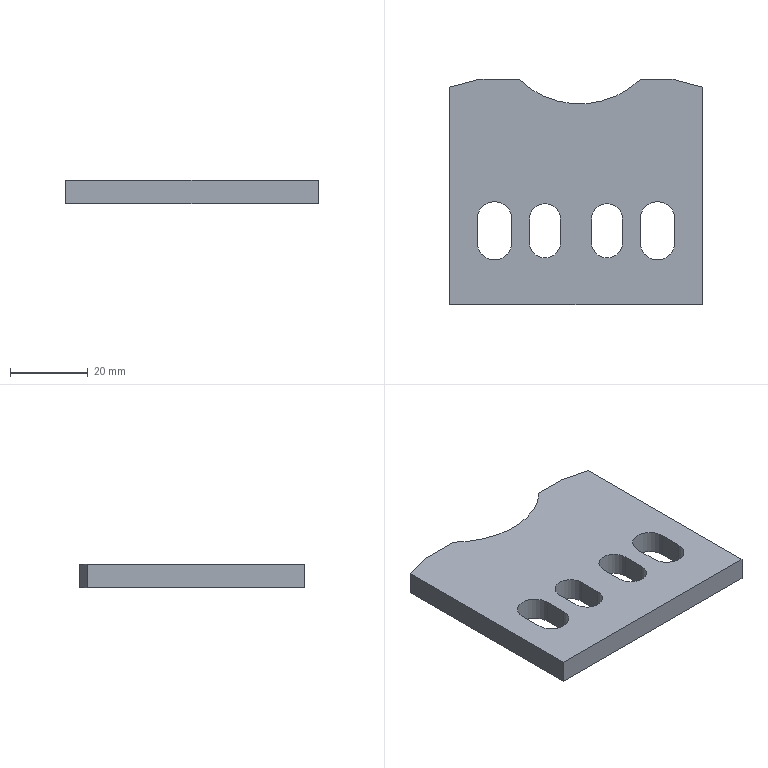Part | STEP file | gslz 2016.10.28-13_id1718_x_t | 1 solid | 26 faces | box 65 x 58 x 6 mm | volume 19127 mm3 | plane 17 | cylinder 9 | commonest cylinder face diameters 8 x4 9 x4 45 x1